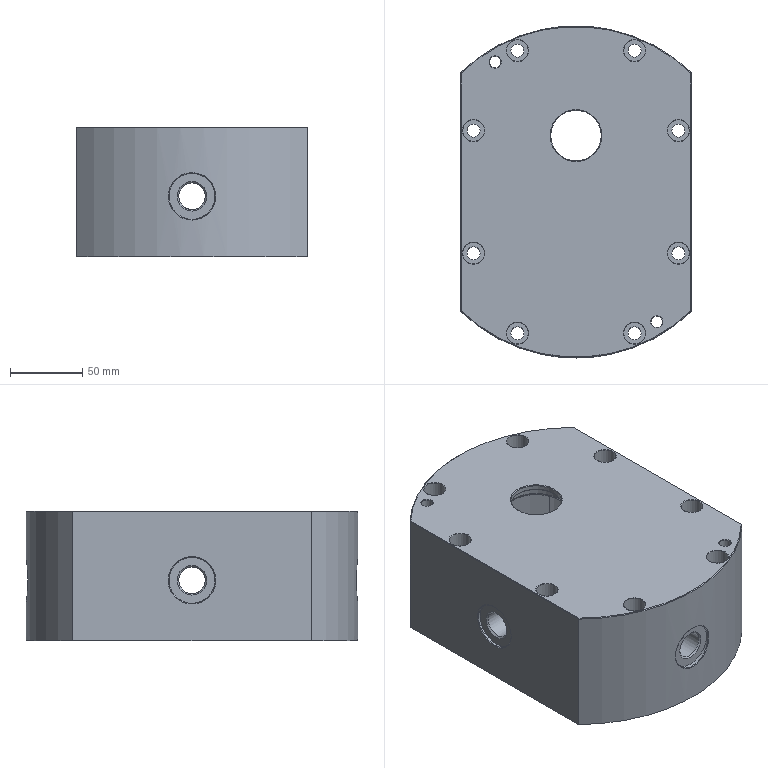NC program | NX | posted with a generic post | part box 160 x 230 x 90 mm
Whole program, first 1056 of 1320 lines:
N10 G17 G21 G94 G90
(HOLE_MILLING_COPY_COPY , TOOL : D10)
N12 T10 M6
N14 G54
N16 G17 G0 G90 X-97.931 Y40.564 B0. C0. S3000 M3
N18 G43 Z30. H10
N20 Z0.5
N22 G94 G3 X-99.181 Y39.314 R1.25 F2200.
N24 X-97.931 Y38.064 R1.25
N26 X-97.931 Y38.064 Z0.28 I0. J2.5
N28 X-97.931 Y38.064 Z0.06 I0. J2.5
N30 X-97.931 Y38.064 Z-0.16 I0. J2.5
N32 X-97.931 Y38.064 Z-0.38 I0. J2.5
N34 X-97.931 Y38.064 Z-0.6 I0. J2.5
N36 X-97.931 Y38.064 Z-0.82 I0. J2.5
N38 X-97.931 Y38.064 Z-1.04 I0. J2.5
N40 X-97.931 Y38.064 Z-1.26 I0. J2.5
N42 X-97.931 Y38.064 Z-1.48 I0. J2.5
N44 X-97.931 Y38.064 Z-1.7 I0. J2.5
N46 X-97.931 Y38.064 Z-1.92 I0. J2.5
N48 X-97.931 Y38.064 Z-2.14 I0. J2.5
N50 X-97.931 Y38.064 Z-2.36 I0. J2.5
N52 X-97.931 Y38.064 Z-2.58 I0. J2.5
N54 X-97.931 Y38.064 Z-2.8 I0. J2.5
N56 X-97.931 Y38.064 Z-3.02 I0. J2.5
N58 X-97.931 Y38.064 Z-3.24 I0. J2.5
N60 X-97.931 Y38.064 Z-3.46 I0. J2.5
N62 X-97.931 Y38.064 Z-3.68 I0. J2.5
N64 X-97.931 Y38.064 Z-3.9 I0. J2.5
N66 X-97.931 Y38.064 Z-4.12 I0. J2.5
N68 X-97.931 Y38.064 Z-4.34 I0. J2.5
N70 X-97.931 Y38.064 Z-4.56 I0. J2.5
N72 X-97.931 Y38.064 Z-4.78 I0. J2.5
N74 X-97.931 Y38.064 Z-5. I0. J2.5
N76 X-97.931 Y38.064 Z-5.22 I0. J2.5
N78 X-97.931 Y38.064 Z-5.44 I0. J2.5
N80 X-97.931 Y38.064 Z-5.66 I0. J2.5
N82 X-97.931 Y38.064 Z-5.88 I0. J2.5
N84 X-97.931 Y38.064 Z-6.1 I0. J2.5
N86 X-97.931 Y38.064 Z-6.32 I0. J2.5
N88 X-97.931 Y38.064 Z-6.54 I0. J2.5
N90 X-97.931 Y38.064 Z-6.76 I0. J2.5
N92 X-97.931 Y38.064 Z-6.98 I0. J2.5
N94 X-97.931 Y38.064 Z-7.2 I0. J2.5
N96 X-97.931 Y38.064 Z-7.42 I0. J2.5
N98 X-97.931 Y38.064 Z-7.64 I0. J2.5
N100 X-97.931 Y38.064 Z-7.86 I0. J2.5
N102 X-97.931 Y38.064 Z-8.08 I0. J2.5
N104 X-97.931 Y38.064 Z-8.3 I0. J2.5
N106 X-97.931 Y38.064 Z-8.52 I0. J2.5
N108 X-97.931 Y38.064 Z-8.74 I0. J2.5
N110 X-97.931 Y38.064 Z-8.96 I0. J2.5
N112 X-97.931 Y38.064 Z-9.18 I0. J2.5
N114 X-97.931 Y38.064 Z-9.4 I0. J2.5
N116 X-97.931 Y38.064 Z-9.62 I0. J2.5
N118 X-97.931 Y38.064 Z-9.84 I0. J2.5
N120 X-97.931 Y38.064 Z-10.06 I0. J2.5
N122 X-97.931 Y38.064 Z-10.28 I0. J2.5
N124 X-97.931 Y38.064 Z-10.5 I0. J2.5
N126 X-97.931 Y38.064 Z-10.72 I0. J2.5
N128 X-97.931 Y38.064 Z-10.94 I0. J2.5
N130 X-97.931 Y38.064 Z-11.16 I0. J2.5
N132 X-97.931 Y38.064 Z-11.38 I0. J2.5
N134 X-97.931 Y38.064 Z-11.6 I0. J2.5
N136 X-97.931 Y38.064 Z-11.82 I0. J2.5
N138 X-97.931 Y38.064 Z-12.04 I0. J2.5
N140 X-97.931 Y38.064 Z-12.26 I0. J2.5
N142 X-97.931 Y38.064 Z-12.48 I0. J2.5
N144 X-97.931 Y38.064 Z-12.7 I0. J2.5
N146 X-97.931 Y38.064 Z-12.92 I0. J2.5
N148 X-97.931 Y38.064 Z-13.14 I0. J2.5
N150 X-97.931 Y38.064 Z-13.36 I0. J2.5
N152 X-97.931 Y38.064 Z-13.58 I0. J2.5
N154 X-97.931 Y38.064 Z-13.8 I0. J2.5
N156 X-97.931 Y38.064 Z-14.02 I0. J2.5
N158 X-97.931 Y38.064 Z-14.24 I0. J2.5
N160 X-97.931 Y38.064 Z-14.46 I0. J2.5
N162 X-97.931 Y38.064 Z-14.68 I0. J2.5
N164 X-97.931 Y38.064 Z-14.9 I0. J2.5
N166 X-97.931 Y38.064 Z-15.12 I0. J2.5
N168 X-97.931 Y38.064 Z-15.34 I0. J2.5
N170 X-97.931 Y38.064 Z-15.56 I0. J2.5
N172 X-97.931 Y38.064 Z-15.78 I0. J2.5
N174 X-97.931 Y38.064 Z-16. I0. J2.5
N176 X-97.931 Y38.064 Z-16.22 I0. J2.5
N178 X-97.931 Y38.064 Z-16.44 I0. J2.5
N180 X-97.931 Y38.064 Z-16.66 I0. J2.5
N182 X-97.931 Y38.064 Z-16.88 I0. J2.5
N184 X-97.931 Y38.064 Z-17.1 I0. J2.5
N186 X-97.931 Y38.064 Z-17.32 I0. J2.5
N188 X-97.931 Y38.064 Z-17.54 I0. J2.5
N190 X-97.931 Y38.064 Z-17.76 I0. J2.5
N192 X-97.931 Y38.064 Z-17.98 I0. J2.5
N194 X-97.931 Y38.064 Z-18.2 I0. J2.5
N196 X-97.931 Y38.064 Z-18.42 I0. J2.5
N198 X-97.931 Y38.064 Z-18.64 I0. J2.5
N200 X-97.931 Y38.064 Z-18.86 I0. J2.5
N202 X-97.931 Y38.064 Z-19.08 I0. J2.5
N204 X-97.931 Y38.064 Z-19.3 I0. J2.5
N206 X-97.931 Y38.064 Z-19.52 I0. J2.5
N208 X-97.931 Y38.064 Z-19.74 I0. J2.5
N210 X-97.931 Y38.064 Z-19.96 I0. J2.5
N212 X-97.931 Y38.064 Z-20.18 I0. J2.5
N214 X-97.931 Y38.064 Z-20.4 I0. J2.5
N216 X-97.931 Y38.064 Z-20.62 I0. J2.5
N218 X-97.931 Y38.064 Z-20.84 I0. J2.5
N220 X-97.931 Y38.064 Z-21.06 I0. J2.5
N222 X-97.931 Y38.064 Z-21.28 I0. J2.5
N224 X-97.931 Y38.064 Z-21.5 I0. J2.5
N226 X-97.931 Y38.064 Z-21.72 I0. J2.5
N228 X-97.931 Y38.064 Z-21.94 I0. J2.5
N230 X-97.931 Y38.064 Z-22.16 I0. J2.5
N232 X-97.931 Y38.064 Z-22.38 I0. J2.5
N234 X-97.931 Y38.064 Z-22.6 I0. J2.5
N236 X-97.931 Y38.064 Z-22.82 I0. J2.5
N238 X-97.931 Y38.064 Z-23.04 I0. J2.5
N240 X-97.931 Y38.064 Z-23.26 I0. J2.5
N242 X-97.931 Y38.064 Z-23.48 I0. J2.5
N244 X-97.931 Y38.064 Z-23.7 I0. J2.5
N246 X-97.931 Y38.064 Z-23.92 I0. J2.5
N248 X-97.931 Y38.064 Z-24.14 I0. J2.5
N250 X-97.931 Y38.064 Z-24.36 I0. J2.5
N252 X-97.931 Y38.064 Z-24.58 I0. J2.5
N254 X-97.931 Y38.064 Z-24.8 I0. J2.5
N256 X-99.283 Y38.461 Z-25. R-2.5
N258 X-95.828 Y39.213 R2.5
N260 X-99.283 Y38.461 R-2.5
N262 X-97.555 Y38.837 R1.25
N264 X-97.931 Y40.564 R1.25
N266 G0 Z30.
N268 X-42.5 Y71.
N270 Z0.5
N272 G3 X-43.75 Y69.75 R1.25
N274 X-42.5 Y68.5 R1.25
N276 X-42.5 Y68.5 Z0.28 I0. J2.5
N278 X-42.5 Y68.5 Z0.06 I0. J2.5
N280 X-42.5 Y68.5 Z-0.16 I0. J2.5
N282 X-42.5 Y68.5 Z-0.38 I0. J2.5
N284 X-42.5 Y68.5 Z-0.6 I0. J2.5
N286 X-42.5 Y68.5 Z-0.82 I0. J2.5
N288 X-42.5 Y68.5 Z-1.04 I0. J2.5
N290 X-42.5 Y68.5 Z-1.26 I0. J2.5
N292 X-42.5 Y68.5 Z-1.48 I0. J2.5
N294 X-42.5 Y68.5 Z-1.7 I0. J2.5
N296 X-42.5 Y68.5 Z-1.92 I0. J2.5
N298 X-42.5 Y68.5 Z-2.14 I0. J2.5
N300 X-42.5 Y68.5 Z-2.36 I0. J2.5
N302 X-42.5 Y68.5 Z-2.58 I0. J2.5
N304 X-42.5 Y68.5 Z-2.8 I0. J2.5
N306 X-42.5 Y68.5 Z-3.02 I0. J2.5
N308 X-42.5 Y68.5 Z-3.24 I0. J2.5
N310 X-42.5 Y68.5 Z-3.46 I0. J2.5
N312 X-42.5 Y68.5 Z-3.68 I0. J2.5
N314 X-42.5 Y68.5 Z-3.9 I0. J2.5
N316 X-42.5 Y68.5 Z-4.12 I0. J2.5
N318 X-42.5 Y68.5 Z-4.34 I0. J2.5
N320 X-42.5 Y68.5 Z-4.56 I0. J2.5
N322 X-42.5 Y68.5 Z-4.78 I0. J2.5
N324 X-42.5 Y68.5 Z-5. I0. J2.5
N326 X-42.5 Y68.5 Z-5.22 I0. J2.5
N328 X-42.5 Y68.5 Z-5.44 I0. J2.5
N330 X-42.5 Y68.5 Z-5.66 I0. J2.5
N332 X-42.5 Y68.5 Z-5.88 I0. J2.5
N334 X-42.5 Y68.5 Z-6.1 I0. J2.5
N336 X-42.5 Y68.5 Z-6.32 I0. J2.5
N338 X-42.5 Y68.5 Z-6.54 I0. J2.5
N340 X-42.5 Y68.5 Z-6.76 I0. J2.5
N342 X-42.5 Y68.5 Z-6.98 I0. J2.5
N344 X-42.5 Y68.5 Z-7.2 I0. J2.5
N346 X-42.5 Y68.5 Z-7.42 I0. J2.5
N348 X-42.5 Y68.5 Z-7.64 I0. J2.5
N350 X-42.5 Y68.5 Z-7.86 I0. J2.5
N352 X-42.5 Y68.5 Z-8.08 I0. J2.5
N354 X-42.5 Y68.5 Z-8.3 I0. J2.5
N356 X-42.5 Y68.5 Z-8.52 I0. J2.5
N358 X-42.5 Y68.5 Z-8.74 I0. J2.5
N360 X-42.5 Y68.5 Z-8.96 I0. J2.5
N362 X-42.5 Y68.5 Z-9.18 I0. J2.5
N364 X-42.5 Y68.5 Z-9.4 I0. J2.5
N366 X-42.5 Y68.5 Z-9.62 I0. J2.5
N368 X-42.5 Y68.5 Z-9.84 I0. J2.5
N370 X-42.5 Y68.5 Z-10.06 I0. J2.5
N372 X-42.5 Y68.5 Z-10.28 I0. J2.5
N374 X-42.5 Y68.5 Z-10.5 I0. J2.5
N376 X-42.5 Y68.5 Z-10.72 I0. J2.5
N378 X-42.5 Y68.5 Z-10.94 I0. J2.5
N380 X-42.5 Y68.5 Z-11.16 I0. J2.5
N382 X-42.5 Y68.5 Z-11.38 I0. J2.5
N384 X-42.5 Y68.5 Z-11.6 I0. J2.5
N386 X-42.5 Y68.5 Z-11.82 I0. J2.5
N388 X-42.5 Y68.5 Z-12.04 I0. J2.5
N390 X-42.5 Y68.5 Z-12.26 I0. J2.5
N392 X-42.5 Y68.5 Z-12.48 I0. J2.5
N394 X-42.5 Y68.5 Z-12.7 I0. J2.5
N396 X-42.5 Y68.5 Z-12.92 I0. J2.5
N398 X-42.5 Y68.5 Z-13.14 I0. J2.5
N400 X-42.5 Y68.5 Z-13.36 I0. J2.5
N402 X-42.5 Y68.5 Z-13.58 I0. J2.5
N404 X-42.5 Y68.5 Z-13.8 I0. J2.5
N406 X-42.5 Y68.5 Z-14.02 I0. J2.5
N408 X-42.5 Y68.5 Z-14.24 I0. J2.5
N410 X-42.5 Y68.5 Z-14.46 I0. J2.5
N412 X-42.5 Y68.5 Z-14.68 I0. J2.5
N414 X-42.5 Y68.5 Z-14.9 I0. J2.5
N416 X-42.5 Y68.5 Z-15.12 I0. J2.5
N418 X-42.5 Y68.5 Z-15.34 I0. J2.5
N420 X-42.5 Y68.5 Z-15.56 I0. J2.5
N422 X-42.5 Y68.5 Z-15.78 I0. J2.5
N424 X-42.5 Y68.5 Z-16. I0. J2.5
N426 X-42.5 Y68.5 Z-16.22 I0. J2.5
N428 X-42.5 Y68.5 Z-16.44 I0. J2.5
N430 X-42.5 Y68.5 Z-16.66 I0. J2.5
N432 X-42.5 Y68.5 Z-16.88 I0. J2.5
N434 X-42.5 Y68.5 Z-17.1 I0. J2.5
N436 X-42.5 Y68.5 Z-17.32 I0. J2.5
N438 X-42.5 Y68.5 Z-17.54 I0. J2.5
N440 X-42.5 Y68.5 Z-17.76 I0. J2.5
N442 X-42.5 Y68.5 Z-17.98 I0. J2.5
N444 X-42.5 Y68.5 Z-18.2 I0. J2.5
N446 X-42.5 Y68.5 Z-18.42 I0. J2.5
N448 X-42.5 Y68.5 Z-18.64 I0. J2.5
N450 X-42.5 Y68.5 Z-18.86 I0. J2.5
N452 X-42.5 Y68.5 Z-19.08 I0. J2.5
N454 X-42.5 Y68.5 Z-19.3 I0. J2.5
N456 X-42.5 Y68.5 Z-19.52 I0. J2.5
N458 X-42.5 Y68.5 Z-19.74 I0. J2.5
N460 X-42.5 Y68.5 Z-19.96 I0. J2.5
N462 X-42.5 Y68.5 Z-20.18 I0. J2.5
N464 X-42.5 Y68.5 Z-20.4 I0. J2.5
N466 X-42.5 Y68.5 Z-20.62 I0. J2.5
N468 X-42.5 Y68.5 Z-20.84 I0. J2.5
N470 X-42.5 Y68.5 Z-21.06 I0. J2.5
N472 X-42.5 Y68.5 Z-21.28 I0. J2.5
N474 X-42.5 Y68.5 Z-21.5 I0. J2.5
N476 X-42.5 Y68.5 Z-21.72 I0. J2.5
N478 X-42.5 Y68.5 Z-21.94 I0. J2.5
N480 X-42.5 Y68.5 Z-22.16 I0. J2.5
N482 X-42.5 Y68.5 Z-22.38 I0. J2.5
N484 X-42.5 Y68.5 Z-22.6 I0. J2.5
N486 X-42.5 Y68.5 Z-22.82 I0. J2.5
N488 X-42.5 Y68.5 Z-23.04 I0. J2.5
N490 X-42.5 Y68.5 Z-23.26 I0. J2.5
N492 X-42.5 Y68.5 Z-23.48 I0. J2.5
N494 X-42.5 Y68.5 Z-23.7 I0. J2.5
N496 X-42.5 Y68.5 Z-23.92 I0. J2.5
N498 X-42.5 Y68.5 Z-24.14 I0. J2.5
N500 X-42.5 Y68.5 Z-24.36 I0. J2.5
N502 X-42.5 Y68.5 Z-24.58 I0. J2.5
N504 X-42.5 Y68.5 Z-24.8 I0. J2.5
N506 X-43.852 Y68.897 Z-25. R-2.5
N508 X-40.397 Y69.648 R2.5
N510 X-43.852 Y68.897 R-2.5
N512 X-42.124 Y69.273 R1.25
N514 X-42.5 Y71. R1.25
N516 G0 Z30.
N518 X42.5
N520 Z0.5
N522 G3 X41.25 Y69.75 R1.25
N524 X42.5 Y68.5 R1.25
N526 X42.5 Y68.5 Z0.28 I0. J2.5
N528 X42.5 Y68.5 Z0.06 I0. J2.5
N530 X42.5 Y68.5 Z-0.16 I0. J2.5
N532 X42.5 Y68.5 Z-0.38 I0. J2.5
N534 X42.5 Y68.5 Z-0.6 I0. J2.5
N536 X42.5 Y68.5 Z-0.82 I0. J2.5
N538 X42.5 Y68.5 Z-1.04 I0. J2.5
N540 X42.5 Y68.5 Z-1.26 I0. J2.5
N542 X42.5 Y68.5 Z-1.48 I0. J2.5
N544 X42.5 Y68.5 Z-1.7 I0. J2.5
N546 X42.5 Y68.5 Z-1.92 I0. J2.5
N548 X42.5 Y68.5 Z-2.14 I0. J2.5
N550 X42.5 Y68.5 Z-2.36 I0. J2.5
N552 X42.5 Y68.5 Z-2.58 I0. J2.5
N554 X42.5 Y68.5 Z-2.8 I0. J2.5
N556 X42.5 Y68.5 Z-3.02 I0. J2.5
N558 X42.5 Y68.5 Z-3.24 I0. J2.5
N560 X42.5 Y68.5 Z-3.46 I0. J2.5
N562 X42.5 Y68.5 Z-3.68 I0. J2.5
N564 X42.5 Y68.5 Z-3.9 I0. J2.5
N566 X42.5 Y68.5 Z-4.12 I0. J2.5
N568 X42.5 Y68.5 Z-4.34 I0. J2.5
N570 X42.5 Y68.5 Z-4.56 I0. J2.5
N572 X42.5 Y68.5 Z-4.78 I0. J2.5
N574 X42.5 Y68.5 Z-5. I0. J2.5
N576 X42.5 Y68.5 Z-5.22 I0. J2.5
N578 X42.5 Y68.5 Z-5.44 I0. J2.5
N580 X42.5 Y68.5 Z-5.66 I0. J2.5
N582 X42.5 Y68.5 Z-5.88 I0. J2.5
N584 X42.5 Y68.5 Z-6.1 I0. J2.5
N586 X42.5 Y68.5 Z-6.32 I0. J2.5
N588 X42.5 Y68.5 Z-6.54 I0. J2.5
N590 X42.5 Y68.5 Z-6.76 I0. J2.5
N592 X42.5 Y68.5 Z-6.98 I0. J2.5
N594 X42.5 Y68.5 Z-7.2 I0. J2.5
N596 X42.5 Y68.5 Z-7.42 I0. J2.5
N598 X42.5 Y68.5 Z-7.64 I0. J2.5
N600 X42.5 Y68.5 Z-7.86 I0. J2.5
N602 X42.5 Y68.5 Z-8.08 I0. J2.5
N604 X42.5 Y68.5 Z-8.3 I0. J2.5
N606 X42.5 Y68.5 Z-8.52 I0. J2.5
N608 X42.5 Y68.5 Z-8.74 I0. J2.5
N610 X42.5 Y68.5 Z-8.96 I0. J2.5
N612 X42.5 Y68.5 Z-9.18 I0. J2.5
N614 X42.5 Y68.5 Z-9.4 I0. J2.5
N616 X42.5 Y68.5 Z-9.62 I0. J2.5
N618 X42.5 Y68.5 Z-9.84 I0. J2.5
N620 X42.5 Y68.5 Z-10.06 I0. J2.5
N622 X42.5 Y68.5 Z-10.28 I0. J2.5
N624 X42.5 Y68.5 Z-10.5 I0. J2.5
N626 X42.5 Y68.5 Z-10.72 I0. J2.5
N628 X42.5 Y68.5 Z-10.94 I0. J2.5
N630 X42.5 Y68.5 Z-11.16 I0. J2.5
N632 X42.5 Y68.5 Z-11.38 I0. J2.5
N634 X42.5 Y68.5 Z-11.6 I0. J2.5
N636 X42.5 Y68.5 Z-11.82 I0. J2.5
N638 X42.5 Y68.5 Z-12.04 I0. J2.5
N640 X42.5 Y68.5 Z-12.26 I0. J2.5
N642 X42.5 Y68.5 Z-12.48 I0. J2.5
N644 X42.5 Y68.5 Z-12.7 I0. J2.5
N646 X42.5 Y68.5 Z-12.92 I0. J2.5
N648 X42.5 Y68.5 Z-13.14 I0. J2.5
N650 X42.5 Y68.5 Z-13.36 I0. J2.5
N652 X42.5 Y68.5 Z-13.58 I0. J2.5
N654 X42.5 Y68.5 Z-13.8 I0. J2.5
N656 X42.5 Y68.5 Z-14.02 I0. J2.5
N658 X42.5 Y68.5 Z-14.24 I0. J2.5
N660 X42.5 Y68.5 Z-14.46 I0. J2.5
N662 X42.5 Y68.5 Z-14.68 I0. J2.5
N664 X42.5 Y68.5 Z-14.9 I0. J2.5
N666 X42.5 Y68.5 Z-15.12 I0. J2.5
N668 X42.5 Y68.5 Z-15.34 I0. J2.5
N670 X42.5 Y68.5 Z-15.56 I0. J2.5
N672 X42.5 Y68.5 Z-15.78 I0. J2.5
N674 X42.5 Y68.5 Z-16. I0. J2.5
N676 X42.5 Y68.5 Z-16.22 I0. J2.5
N678 X42.5 Y68.5 Z-16.44 I0. J2.5
N680 X42.5 Y68.5 Z-16.66 I0. J2.5
N682 X42.5 Y68.5 Z-16.88 I0. J2.5
N684 X42.5 Y68.5 Z-17.1 I0. J2.5
N686 X42.5 Y68.5 Z-17.32 I0. J2.5
N688 X42.5 Y68.5 Z-17.54 I0. J2.5
N690 X42.5 Y68.5 Z-17.76 I0. J2.5
N692 X42.5 Y68.5 Z-17.98 I0. J2.5
N694 X42.5 Y68.5 Z-18.2 I0. J2.5
N696 X42.5 Y68.5 Z-18.42 I0. J2.5
N698 X42.5 Y68.5 Z-18.64 I0. J2.5
N700 X42.5 Y68.5 Z-18.86 I0. J2.5
N702 X42.5 Y68.5 Z-19.08 I0. J2.5
N704 X42.5 Y68.5 Z-19.3 I0. J2.5
N706 X42.5 Y68.5 Z-19.52 I0. J2.5
N708 X42.5 Y68.5 Z-19.74 I0. J2.5
N710 X42.5 Y68.5 Z-19.96 I0. J2.5
N712 X42.5 Y68.5 Z-20.18 I0. J2.5
N714 X42.5 Y68.5 Z-20.4 I0. J2.5
N716 X42.5 Y68.5 Z-20.62 I0. J2.5
N718 X42.5 Y68.5 Z-20.84 I0. J2.5
N720 X42.5 Y68.5 Z-21.06 I0. J2.5
N722 X42.5 Y68.5 Z-21.28 I0. J2.5
N724 X42.5 Y68.5 Z-21.5 I0. J2.5
N726 X42.5 Y68.5 Z-21.72 I0. J2.5
N728 X42.5 Y68.5 Z-21.94 I0. J2.5
N730 X42.5 Y68.5 Z-22.16 I0. J2.5
N732 X42.5 Y68.5 Z-22.38 I0. J2.5
N734 X42.5 Y68.5 Z-22.6 I0. J2.5
N736 X42.5 Y68.5 Z-22.82 I0. J2.5
N738 X42.5 Y68.5 Z-23.04 I0. J2.5
N740 X42.5 Y68.5 Z-23.26 I0. J2.5
N742 X42.5 Y68.5 Z-23.48 I0. J2.5
N744 X42.5 Y68.5 Z-23.7 I0. J2.5
N746 X42.5 Y68.5 Z-23.92 I0. J2.5
N748 X42.5 Y68.5 Z-24.14 I0. J2.5
N750 X42.5 Y68.5 Z-24.36 I0. J2.5
N752 X42.5 Y68.5 Z-24.58 I0. J2.5
N754 X42.5 Y68.5 Z-24.8 I0. J2.5
N756 X41.148 Y68.897 Z-25. R-2.5
N758 X44.603 Y69.648 R2.5
N760 X41.148 Y68.897 R-2.5
N762 X42.876 Y69.273 R1.25
N764 X42.5 Y71. R1.25
N766 G0 Z30.
N768 X97.931 Y40.564
N770 Z0.5
N772 G3 X96.681 Y39.314 R1.25
N774 X97.931 Y38.064 R1.25
N776 X97.931 Y38.064 Z0.28 I0. J2.5
N778 X97.931 Y38.064 Z0.06 I0. J2.5
N780 X97.931 Y38.064 Z-0.16 I0. J2.5
N782 X97.931 Y38.064 Z-0.38 I0. J2.5
N784 X97.931 Y38.064 Z-0.6 I0. J2.5
N786 X97.931 Y38.064 Z-0.82 I0. J2.5
N788 X97.931 Y38.064 Z-1.04 I0. J2.5
N790 X97.931 Y38.064 Z-1.26 I0. J2.5
N792 X97.931 Y38.064 Z-1.48 I0. J2.5
N794 X97.931 Y38.064 Z-1.7 I0. J2.5
N796 X97.931 Y38.064 Z-1.92 I0. J2.5
N798 X97.931 Y38.064 Z-2.14 I0. J2.5
N800 X97.931 Y38.064 Z-2.36 I0. J2.5
N802 X97.931 Y38.064 Z-2.58 I0. J2.5
N804 X97.931 Y38.064 Z-2.8 I0. J2.5
N806 X97.931 Y38.064 Z-3.02 I0. J2.5
N808 X97.931 Y38.064 Z-3.24 I0. J2.5
N810 X97.931 Y38.064 Z-3.46 I0. J2.5
N812 X97.931 Y38.064 Z-3.68 I0. J2.5
N814 X97.931 Y38.064 Z-3.9 I0. J2.5
N816 X97.931 Y38.064 Z-4.12 I0. J2.5
N818 X97.931 Y38.064 Z-4.34 I0. J2.5
N820 X97.931 Y38.064 Z-4.56 I0. J2.5
N822 X97.931 Y38.064 Z-4.78 I0. J2.5
N824 X97.931 Y38.064 Z-5. I0. J2.5
N826 X97.931 Y38.064 Z-5.22 I0. J2.5
N828 X97.931 Y38.064 Z-5.44 I0. J2.5
N830 X97.931 Y38.064 Z-5.66 I0. J2.5
N832 X97.931 Y38.064 Z-5.88 I0. J2.5
N834 X97.931 Y38.064 Z-6.1 I0. J2.5
N836 X97.931 Y38.064 Z-6.32 I0. J2.5
N838 X97.931 Y38.064 Z-6.54 I0. J2.5
N840 X97.931 Y38.064 Z-6.76 I0. J2.5
N842 X97.931 Y38.064 Z-6.98 I0. J2.5
N844 X97.931 Y38.064 Z-7.2 I0. J2.5
N846 X97.931 Y38.064 Z-7.42 I0. J2.5
N848 X97.931 Y38.064 Z-7.64 I0. J2.5
N850 X97.931 Y38.064 Z-7.86 I0. J2.5
N852 X97.931 Y38.064 Z-8.08 I0. J2.5
N854 X97.931 Y38.064 Z-8.3 I0. J2.5
N856 X97.931 Y38.064 Z-8.52 I0. J2.5
N858 X97.931 Y38.064 Z-8.74 I0. J2.5
N860 X97.931 Y38.064 Z-8.96 I0. J2.5
N862 X97.931 Y38.064 Z-9.18 I0. J2.5
N864 X97.931 Y38.064 Z-9.4 I0. J2.5
N866 X97.931 Y38.064 Z-9.62 I0. J2.5
N868 X97.931 Y38.064 Z-9.84 I0. J2.5
N870 X97.931 Y38.064 Z-10.06 I0. J2.5
N872 X97.931 Y38.064 Z-10.28 I0. J2.5
N874 X97.931 Y38.064 Z-10.5 I0. J2.5
N876 X97.931 Y38.064 Z-10.72 I0. J2.5
N878 X97.931 Y38.064 Z-10.94 I0. J2.5
N880 X97.931 Y38.064 Z-11.16 I0. J2.5
N882 X97.931 Y38.064 Z-11.38 I0. J2.5
N884 X97.931 Y38.064 Z-11.6 I0. J2.5
N886 X97.931 Y38.064 Z-11.82 I0. J2.5
N888 X97.931 Y38.064 Z-12.04 I0. J2.5
N890 X97.931 Y38.064 Z-12.26 I0. J2.5
N892 X97.931 Y38.064 Z-12.48 I0. J2.5
N894 X97.931 Y38.064 Z-12.7 I0. J2.5
N896 X97.931 Y38.064 Z-12.92 I0. J2.5
N898 X97.931 Y38.064 Z-13.14 I0. J2.5
N900 X97.931 Y38.064 Z-13.36 I0. J2.5
N902 X97.931 Y38.064 Z-13.58 I0. J2.5
N904 X97.931 Y38.064 Z-13.8 I0. J2.5
N906 X97.931 Y38.064 Z-14.02 I0. J2.5
N908 X97.931 Y38.064 Z-14.24 I0. J2.5
N910 X97.931 Y38.064 Z-14.46 I0. J2.5
N912 X97.931 Y38.064 Z-14.68 I0. J2.5
N914 X97.931 Y38.064 Z-14.9 I0. J2.5
N916 X97.931 Y38.064 Z-15.12 I0. J2.5
N918 X97.931 Y38.064 Z-15.34 I0. J2.5
N920 X97.931 Y38.064 Z-15.56 I0. J2.5
N922 X97.931 Y38.064 Z-15.78 I0. J2.5
N924 X97.931 Y38.064 Z-16. I0. J2.5
N926 X97.931 Y38.064 Z-16.22 I0. J2.5
N928 X97.931 Y38.064 Z-16.44 I0. J2.5
N930 X97.931 Y38.064 Z-16.66 I0. J2.5
N932 X97.931 Y38.064 Z-16.88 I0. J2.5
N934 X97.931 Y38.064 Z-17.1 I0. J2.5
N936 X97.931 Y38.064 Z-17.32 I0. J2.5
N938 X97.931 Y38.064 Z-17.54 I0. J2.5
N940 X97.931 Y38.064 Z-17.76 I0. J2.5
N942 X97.931 Y38.064 Z-17.98 I0. J2.5
N944 X97.931 Y38.064 Z-18.2 I0. J2.5
N946 X97.931 Y38.064 Z-18.42 I0. J2.5
N948 X97.931 Y38.064 Z-18.64 I0. J2.5
N950 X97.931 Y38.064 Z-18.86 I0. J2.5
N952 X97.931 Y38.064 Z-19.08 I0. J2.5
N954 X97.931 Y38.064 Z-19.3 I0. J2.5
N956 X97.931 Y38.064 Z-19.52 I0. J2.5
N958 X97.931 Y38.064 Z-19.74 I0. J2.5
N960 X97.931 Y38.064 Z-19.96 I0. J2.5
N962 X97.931 Y38.064 Z-20.18 I0. J2.5
N964 X97.931 Y38.064 Z-20.4 I0. J2.5
N966 X97.931 Y38.064 Z-20.62 I0. J2.5
N968 X97.931 Y38.064 Z-20.84 I0. J2.5
N970 X97.931 Y38.064 Z-21.06 I0. J2.5
N972 X97.931 Y38.064 Z-21.28 I0. J2.5
N974 X97.931 Y38.064 Z-21.5 I0. J2.5
N976 X97.931 Y38.064 Z-21.72 I0. J2.5
N978 X97.931 Y38.064 Z-21.94 I0. J2.5
N980 X97.931 Y38.064 Z-22.16 I0. J2.5
N982 X97.931 Y38.064 Z-22.38 I0. J2.5
N984 X97.931 Y38.064 Z-22.6 I0. J2.5
N986 X97.931 Y38.064 Z-22.82 I0. J2.5
N988 X97.931 Y38.064 Z-23.04 I0. J2.5
N990 X97.931 Y38.064 Z-23.26 I0. J2.5
N992 X97.931 Y38.064 Z-23.48 I0. J2.5
N994 X97.931 Y38.064 Z-23.7 I0. J2.5
N996 X97.931 Y38.064 Z-23.92 I0. J2.5
N998 X97.931 Y38.064 Z-24.14 I0. J2.5
N1000 X97.931 Y38.064 Z-24.36 I0. J2.5
N1002 X97.931 Y38.064 Z-24.58 I0. J2.5
N1004 X97.931 Y38.064 Z-24.8 I0. J2.5
N1006 X96.58 Y38.461 Z-25. R-2.5
N1008 X100.034 Y39.213 R2.5
N1010 X96.58 Y38.461 R-2.5
N1012 X98.307 Y38.837 R1.25
N1014 X97.931 Y40.564 R1.25
N1016 G0 Z30.
N1018 Y-40.564
N1020 Z0.5
N1022 G3 X96.681 Y-41.814 R1.25
N1024 X97.931 Y-43.064 R1.25
N1026 X97.931 Y-43.064 Z0.28 I0. J2.5
N1028 X97.931 Y-43.064 Z0.06 I0. J2.5
N1030 X97.931 Y-43.064 Z-0.16 I0. J2.5
N1032 X97.931 Y-43.064 Z-0.38 I0. J2.5
N1034 X97.931 Y-43.064 Z-0.6 I0. J2.5
N1036 X97.931 Y-43.064 Z-0.82 I0. J2.5
N1038 X97.931 Y-43.064 Z-1.04 I0. J2.5
N1040 X97.931 Y-43.064 Z-1.26 I0. J2.5
N1042 X97.931 Y-43.064 Z-1.48 I0. J2.5
N1044 X97.931 Y-43.064 Z-1.7 I0. J2.5
N1046 X97.931 Y-43.064 Z-1.92 I0. J2.5
N1048 X97.931 Y-43.064 Z-2.14 I0. J2.5
N1050 X97.931 Y-43.064 Z-2.36 I0. J2.5
N1052 X97.931 Y-43.064 Z-2.58 I0. J2.5
N1054 X97.931 Y-43.064 Z-2.8 I0. J2.5
N1056 X97.931 Y-43.064 Z-3.02 I0. J2.5
N1058 X97.931 Y-43.064 Z-3.24 I0. J2.5
N1060 X97.931 Y-43.064 Z-3.46 I0. J2.5
N1062 X97.931 Y-43.064 Z-3.68 I0. J2.5
N1064 X97.931 Y-43.064 Z-3.9 I0. J2.5
N1066 X97.931 Y-43.064 Z-4.12 I0. J2.5
N1068 X97.931 Y-43.064 Z-4.34 I0. J2.5
N1070 X97.931 Y-43.064 Z-4.56 I0. J2.5
N1072 X97.931 Y-43.064 Z-4.78 I0. J2.5
N1074 X97.931 Y-43.064 Z-5. I0. J2.5
N1076 X97.931 Y-43.064 Z-5.22 I0. J2.5
N1078 X97.931 Y-43.064 Z-5.44 I0. J2.5
N1080 X97.931 Y-43.064 Z-5.66 I0. J2.5
N1082 X97.931 Y-43.064 Z-5.88 I0. J2.5
N1084 X97.931 Y-43.064 Z-6.1 I0. J2.5
N1086 X97.931 Y-43.064 Z-6.32 I0. J2.5
N1088 X97.931 Y-43.064 Z-6.54 I0. J2.5
N1090 X97.931 Y-43.064 Z-6.76 I0. J2.5
N1092 X97.931 Y-43.064 Z-6.98 I0. J2.5
N1094 X97.931 Y-43.064 Z-7.2 I0. J2.5
N1096 X97.931 Y-43.064 Z-7.42 I0. J2.5
N1098 X97.931 Y-43.064 Z-7.64 I0. J2.5
N1100 X97.931 Y-43.064 Z-7.86 I0. J2.5
N1102 X97.931 Y-43.064 Z-8.08 I0. J2.5
N1104 X97.931 Y-43.064 Z-8.3 I0. J2.5
N1106 X97.931 Y-43.064 Z-8.52 I0. J2.5
N1108 X97.931 Y-43.064 Z-8.74 I0. J2.5
N1110 X97.931 Y-43.064 Z-8.96 I0. J2.5
N1112 X97.931 Y-43.064 Z-9.18 I0. J2.5
N1114 X97.931 Y-43.064 Z-9.4 I0. J2.5
N1116 X97.931 Y-43.064 Z-9.62 I0. J2.5
N1118 X97.931 Y-43.064 Z-9.84 I0. J2.5
N1120 X97.931 Y-43.064 Z-10.06 I0. J2.5
N1122 X97.931 Y-43.064 Z-10.28 I0. J2.5
N1124 X97.931 Y-43.064 Z-10.5 I0. J2.5
N1126 X97.931 Y-43.064 Z-10.72 I0. J2.5
N1128 X97.931 Y-43.064 Z-10.94 I0. J2.5
N1130 X97.931 Y-43.064 Z-11.16 I0. J2.5
N1132 X97.931 Y-43.064 Z-11.38 I0. J2.5
N1134 X97.931 Y-43.064 Z-11.6 I0. J2.5
N1136 X97.931 Y-43.064 Z-11.82 I0. J2.5
N1138 X97.931 Y-43.064 Z-12.04 I0. J2.5
N1140 X97.931 Y-43.064 Z-12.26 I0. J2.5
N1142 X97.931 Y-43.064 Z-12.48 I0. J2.5
N1144 X97.931 Y-43.064 Z-12.7 I0. J2.5
N1146 X97.931 Y-43.064 Z-12.92 I0. J2.5
N1148 X97.931 Y-43.064 Z-13.14 I0. J2.5
N1150 X97.931 Y-43.064 Z-13.36 I0. J2.5
N1152 X97.931 Y-43.064 Z-13.58 I0. J2.5
N1154 X97.931 Y-43.064 Z-13.8 I0. J2.5
N1156 X97.931 Y-43.064 Z-14.02 I0. J2.5
N1158 X97.931 Y-43.064 Z-14.24 I0. J2.5
N1160 X97.931 Y-43.064 Z-14.46 I0. J2.5
N1162 X97.931 Y-43.064 Z-14.68 I0. J2.5
N1164 X97.931 Y-43.064 Z-14.9 I0. J2.5
N1166 X97.931 Y-43.064 Z-15.12 I0. J2.5
N1168 X97.931 Y-43.064 Z-15.34 I0. J2.5
N1170 X97.931 Y-43.064 Z-15.56 I0. J2.5
N1172 X97.931 Y-43.064 Z-15.78 I0. J2.5
N1174 X97.931 Y-43.064 Z-16. I0. J2.5
N1176 X97.931 Y-43.064 Z-16.22 I0. J2.5
N1178 X97.931 Y-43.064 Z-16.44 I0. J2.5
N1180 X97.931 Y-43.064 Z-16.66 I0. J2.5
N1182 X97.931 Y-43.064 Z-16.88 I0. J2.5
N1184 X97.931 Y-43.064 Z-17.1 I0. J2.5
N1186 X97.931 Y-43.064 Z-17.32 I0. J2.5
N1188 X97.931 Y-43.064 Z-17.54 I0. J2.5
N1190 X97.931 Y-43.064 Z-17.76 I0. J2.5
N1192 X97.931 Y-43.064 Z-17.98 I0. J2.5
N1194 X97.931 Y-43.064 Z-18.2 I0. J2.5
N1196 X97.931 Y-43.064 Z-18.42 I0. J2.5
N1198 X97.931 Y-43.064 Z-18.64 I0. J2.5
N1200 X97.931 Y-43.064 Z-18.86 I0. J2.5
N1202 X97.931 Y-43.064 Z-19.08 I0. J2.5
N1204 X97.931 Y-43.064 Z-19.3 I0. J2.5
N1206 X97.931 Y-43.064 Z-19.52 I0. J2.5
N1208 X97.931 Y-43.064 Z-19.74 I0. J2.5
N1210 X97.931 Y-43.064 Z-19.96 I0. J2.5
N1212 X97.931 Y-43.064 Z-20.18 I0. J2.5
N1214 X97.931 Y-43.064 Z-20.4 I0. J2.5
N1216 X97.931 Y-43.064 Z-20.62 I0. J2.5
N1218 X97.931 Y-43.064 Z-20.84 I0. J2.5
N1220 X97.931 Y-43.064 Z-21.06 I0. J2.5
N1222 X97.931 Y-43.064 Z-21.28 I0. J2.5
N1224 X97.931 Y-43.064 Z-21.5 I0. J2.5
N1226 X97.931 Y-43.064 Z-21.72 I0. J2.5
N1228 X97.931 Y-43.064 Z-21.94 I0. J2.5
N1230 X97.931 Y-43.064 Z-22.16 I0. J2.5
N1232 X97.931 Y-43.064 Z-22.38 I0. J2.5
N1234 X97.931 Y-43.064 Z-22.6 I0. J2.5
N1236 X97.931 Y-43.064 Z-22.82 I0. J2.5
N1238 X97.931 Y-43.064 Z-23.04 I0. J2.5
N1240 X97.931 Y-43.064 Z-23.26 I0. J2.5
N1242 X97.931 Y-43.064 Z-23.48 I0. J2.5
N1244 X97.931 Y-43.064 Z-23.7 I0. J2.5
N1246 X97.931 Y-43.064 Z-23.92 I0. J2.5
N1248 X97.931 Y-43.064 Z-24.14 I0. J2.5
N1250 X97.931 Y-43.064 Z-24.36 I0. J2.5
N1252 X97.931 Y-43.064 Z-24.58 I0. J2.5
N1254 X97.931 Y-43.064 Z-24.8 I0. J2.5
N1256 X96.58 Y-42.668 Z-25. R-2.5
N1258 X100.034 Y-41.916 R2.5
N1260 X96.58 Y-42.668 R-2.5
N1262 X98.307 Y-42.292 R1.25
N1264 X97.931 Y-40.564 R1.25
N1266 G0 Z30.
N1268 X42.5 Y-71.
N1270 Z0.5
N1272 G3 X41.25 Y-72.25 R1.25
N1274 X42.5 Y-73.5 R1.25
N1276 X42.5 Y-73.5 Z0.28 I0. J2.5
N1278 X42.5 Y-73.5 Z0.06 I0. J2.5
N1280 X42.5 Y-73.5 Z-0.16 I0. J2.5
N1282 X42.5 Y-73.5 Z-0.38 I0. J2.5
N1284 X42.5 Y-73.5 Z-0.6 I0. J2.5
N1286 X42.5 Y-73.5 Z-0.82 I0. J2.5
N1288 X42.5 Y-73.5 Z-1.04 I0. J2.5
N1290 X42.5 Y-73.5 Z-1.26 I0. J2.5
N1292 X42.5 Y-73.5 Z-1.48 I0. J2.5
N1294 X42.5 Y-73.5 Z-1.7 I0. J2.5
N1296 X42.5 Y-73.5 Z-1.92 I0. J2.5
N1298 X42.5 Y-73.5 Z-2.14 I0. J2.5
N1300 X42.5 Y-73.5 Z-2.36 I0. J2.5
N1302 X42.5 Y-73.5 Z-2.58 I0. J2.5
N1304 X42.5 Y-73.5 Z-2.8 I0. J2.5
N1306 X42.5 Y-73.5 Z-3.02 I0. J2.5
N1308 X42.5 Y-73.5 Z-3.24 I0. J2.5
N1310 X42.5 Y-73.5 Z-3.46 I0. J2.5
N1312 X42.5 Y-73.5 Z-3.68 I0. J2.5
N1314 X42.5 Y-73.5 Z-3.9 I0. J2.5
N1316 X42.5 Y-73.5 Z-4.12 I0. J2.5
N1318 X42.5 Y-73.5 Z-4.34 I0. J2.5
N1320 X42.5 Y-73.5 Z-4.56 I0. J2.5
N1322 X42.5 Y-73.5 Z-4.78 I0. J2.5
N1324 X42.5 Y-73.5 Z-5. I0. J2.5
N1326 X42.5 Y-73.5 Z-5.22 I0. J2.5
N1328 X42.5 Y-73.5 Z-5.44 I0. J2.5
N1330 X42.5 Y-73.5 Z-5.66 I0. J2.5
N1332 X42.5 Y-73.5 Z-5.88 I0. J2.5
N1334 X42.5 Y-73.5 Z-6.1 I0. J2.5
N1336 X42.5 Y-73.5 Z-6.32 I0. J2.5
N1338 X42.5 Y-73.5 Z-6.54 I0. J2.5
N1340 X42.5 Y-73.5 Z-6.76 I0. J2.5
N1342 X42.5 Y-73.5 Z-6.98 I0. J2.5
N1344 X42.5 Y-73.5 Z-7.2 I0. J2.5
N1346 X42.5 Y-73.5 Z-7.42 I0. J2.5
N1348 X42.5 Y-73.5 Z-7.64 I0. J2.5
N1350 X42.5 Y-73.5 Z-7.86 I0. J2.5
N1352 X42.5 Y-73.5 Z-8.08 I0. J2.5
N1354 X42.5 Y-73.5 Z-8.3 I0. J2.5
N1356 X42.5 Y-73.5 Z-8.52 I0. J2.5
N1358 X42.5 Y-73.5 Z-8.74 I0. J2.5
N1360 X42.5 Y-73.5 Z-8.96 I0. J2.5
N1362 X42.5 Y-73.5 Z-9.18 I0. J2.5
N1364 X42.5 Y-73.5 Z-9.4 I0. J2.5
N1366 X42.5 Y-73.5 Z-9.62 I0. J2.5
N1368 X42.5 Y-73.5 Z-9.84 I0. J2.5
N1370 X42.5 Y-73.5 Z-10.06 I0. J2.5
N1372 X42.5 Y-73.5 Z-10.28 I0. J2.5
N1374 X42.5 Y-73.5 Z-10.5 I0. J2.5
N1376 X42.5 Y-73.5 Z-10.72 I0. J2.5
N1378 X42.5 Y-73.5 Z-10.94 I0. J2.5
N1380 X42.5 Y-73.5 Z-11.16 I0. J2.5
N1382 X42.5 Y-73.5 Z-11.38 I0. J2.5
N1384 X42.5 Y-73.5 Z-11.6 I0. J2.5
N1386 X42.5 Y-73.5 Z-11.82 I0. J2.5
N1388 X42.5 Y-73.5 Z-12.04 I0. J2.5
N1390 X42.5 Y-73.5 Z-12.26 I0. J2.5
N1392 X42.5 Y-73.5 Z-12.48 I0. J2.5
N1394 X42.5 Y-73.5 Z-12.7 I0. J2.5
N1396 X42.5 Y-73.5 Z-12.92 I0. J2.5
N1398 X42.5 Y-73.5 Z-13.14 I0. J2.5
N1400 X42.5 Y-73.5 Z-13.36 I0. J2.5
N1402 X42.5 Y-73.5 Z-13.58 I0. J2.5
N1404 X42.5 Y-73.5 Z-13.8 I0. J2.5
N1406 X42.5 Y-73.5 Z-14.02 I0. J2.5
N1408 X42.5 Y-73.5 Z-14.24 I0. J2.5
N1410 X42.5 Y-73.5 Z-14.46 I0. J2.5
N1412 X42.5 Y-73.5 Z-14.68 I0. J2.5
N1414 X42.5 Y-73.5 Z-14.9 I0. J2.5
N1416 X42.5 Y-73.5 Z-15.12 I0. J2.5
N1418 X42.5 Y-73.5 Z-15.34 I0. J2.5
N1420 X42.5 Y-73.5 Z-15.56 I0. J2.5
N1422 X42.5 Y-73.5 Z-15.78 I0. J2.5
N1424 X42.5 Y-73.5 Z-16. I0. J2.5
N1426 X42.5 Y-73.5 Z-16.22 I0. J2.5
N1428 X42.5 Y-73.5 Z-16.44 I0. J2.5
N1430 X42.5 Y-73.5 Z-16.66 I0. J2.5
N1432 X42.5 Y-73.5 Z-16.88 I0. J2.5
N1434 X42.5 Y-73.5 Z-17.1 I0. J2.5
N1436 X42.5 Y-73.5 Z-17.32 I0. J2.5
N1438 X42.5 Y-73.5 Z-17.54 I0. J2.5
N1440 X42.5 Y-73.5 Z-17.76 I0. J2.5
N1442 X42.5 Y-73.5 Z-17.98 I0. J2.5
N1444 X42.5 Y-73.5 Z-18.2 I0. J2.5
N1446 X42.5 Y-73.5 Z-18.42 I0. J2.5
N1448 X42.5 Y-73.5 Z-18.64 I0. J2.5
N1450 X42.5 Y-73.5 Z-18.86 I0. J2.5
N1452 X42.5 Y-73.5 Z-19.08 I0. J2.5
N1454 X42.5 Y-73.5 Z-19.3 I0. J2.5
N1456 X42.5 Y-73.5 Z-19.52 I0. J2.5
N1458 X42.5 Y-73.5 Z-19.74 I0. J2.5
N1460 X42.5 Y-73.5 Z-19.96 I0. J2.5
N1462 X42.5 Y-73.5 Z-20.18 I0. J2.5
N1464 X42.5 Y-73.5 Z-20.4 I0. J2.5
N1466 X42.5 Y-73.5 Z-20.62 I0. J2.5
N1468 X42.5 Y-73.5 Z-20.84 I0. J2.5
N1470 X42.5 Y-73.5 Z-21.06 I0. J2.5
N1472 X42.5 Y-73.5 Z-21.28 I0. J2.5
N1474 X42.5 Y-73.5 Z-21.5 I0. J2.5
N1476 X42.5 Y-73.5 Z-21.72 I0. J2.5
N1478 X42.5 Y-73.5 Z-21.94 I0. J2.5
N1480 X42.5 Y-73.5 Z-22.16 I0. J2.5
N1482 X42.5 Y-73.5 Z-22.38 I0. J2.5
N1484 X42.5 Y-73.5 Z-22.6 I0. J2.5
N1486 X42.5 Y-73.5 Z-22.82 I0. J2.5
N1488 X42.5 Y-73.5 Z-23.04 I0. J2.5
N1490 X42.5 Y-73.5 Z-23.26 I0. J2.5
N1492 X42.5 Y-73.5 Z-23.48 I0. J2.5
N1494 X42.5 Y-73.5 Z-23.7 I0. J2.5
N1496 X42.5 Y-73.5 Z-23.92 I0. J2.5
N1498 X42.5 Y-73.5 Z-24.14 I0. J2.5
N1500 X42.5 Y-73.5 Z-24.36 I0. J2.5
N1502 X42.5 Y-73.5 Z-24.58 I0. J2.5
N1504 X42.5 Y-73.5 Z-24.8 I0. J2.5
N1506 X41.148 Y-73.103 Z-25. R-2.5
N1508 X44.603 Y-72.352 R2.5
N1510 X41.148 Y-73.103 R-2.5
N1512 X42.876 Y-72.727 R1.25
N1514 X42.5 Y-71. R1.25
N1516 G0 Z30.
N1518 X-42.5
N1520 Z0.5
N1522 G3 X-43.75 Y-72.25 R1.25
N1524 X-42.5 Y-73.5 R1.25
N1526 X-42.5 Y-73.5 Z0.28 I0. J2.5
N1528 X-42.5 Y-73.5 Z0.06 I0. J2.5
N1530 X-42.5 Y-73.5 Z-0.16 I0. J2.5
N1532 X-42.5 Y-73.5 Z-0.38 I0. J2.5
N1534 X-42.5 Y-73.5 Z-0.6 I0. J2.5
N1536 X-42.5 Y-73.5 Z-0.82 I0. J2.5
N1538 X-42.5 Y-73.5 Z-1.04 I0. J2.5
N1540 X-42.5 Y-73.5 Z-1.26 I0. J2.5
N1542 X-42.5 Y-73.5 Z-1.48 I0. J2.5
N1544 X-42.5 Y-73.5 Z-1.7 I0. J2.5
N1546 X-42.5 Y-73.5 Z-1.92 I0. J2.5
N1548 X-42.5 Y-73.5 Z-2.14 I0. J2.5
N1550 X-42.5 Y-73.5 Z-2.36 I0. J2.5
N1552 X-42.5 Y-73.5 Z-2.58 I0. J2.5
N1554 X-42.5 Y-73.5 Z-2.8 I0. J2.5
N1556 X-42.5 Y-73.5 Z-3.02 I0. J2.5
N1558 X-42.5 Y-73.5 Z-3.24 I0. J2.5
N1560 X-42.5 Y-73.5 Z-3.46 I0. J2.5
N1562 X-42.5 Y-73.5 Z-3.68 I0. J2.5
N1564 X-42.5 Y-73.5 Z-3.9 I0. J2.5
N1566 X-42.5 Y-73.5 Z-4.12 I0. J2.5
N1568 X-42.5 Y-73.5 Z-4.34 I0. J2.5
N1570 X-42.5 Y-73.5 Z-4.56 I0. J2.5
N1572 X-42.5 Y-73.5 Z-4.78 I0. J2.5
N1574 X-42.5 Y-73.5 Z-5. I0. J2.5
N1576 X-42.5 Y-73.5 Z-5.22 I0. J2.5
N1578 X-42.5 Y-73.5 Z-5.44 I0. J2.5
N1580 X-42.5 Y-73.5 Z-5.66 I0. J2.5
N1582 X-42.5 Y-73.5 Z-5.88 I0. J2.5
N1584 X-42.5 Y-73.5 Z-6.1 I0. J2.5
N1586 X-42.5 Y-73.5 Z-6.32 I0. J2.5
N1588 X-42.5 Y-73.5 Z-6.54 I0. J2.5
N1590 X-42.5 Y-73.5 Z-6.76 I0. J2.5
N1592 X-42.5 Y-73.5 Z-6.98 I0. J2.5
N1594 X-42.5 Y-73.5 Z-7.2 I0. J2.5
N1596 X-42.5 Y-73.5 Z-7.42 I0. J2.5
N1598 X-42.5 Y-73.5 Z-7.64 I0. J2.5
N1600 X-42.5 Y-73.5 Z-7.86 I0. J2.5
N1602 X-42.5 Y-73.5 Z-8.08 I0. J2.5
N1604 X-42.5 Y-73.5 Z-8.3 I0. J2.5
N1606 X-42.5 Y-73.5 Z-8.52 I0. J2.5
N1608 X-42.5 Y-73.5 Z-8.74 I0. J2.5
N1610 X-42.5 Y-73.5 Z-8.96 I0. J2.5
N1612 X-42.5 Y-73.5 Z-9.18 I0. J2.5
N1614 X-42.5 Y-73.5 Z-9.4 I0. J2.5
N1616 X-42.5 Y-73.5 Z-9.62 I0. J2.5
N1618 X-42.5 Y-73.5 Z-9.84 I0. J2.5
N1620 X-42.5 Y-73.5 Z-10.06 I0. J2.5
N1622 X-42.5 Y-73.5 Z-10.28 I0. J2.5
N1624 X-42.5 Y-73.5 Z-10.5 I0. J2.5
N1626 X-42.5 Y-73.5 Z-10.72 I0. J2.5
N1628 X-42.5 Y-73.5 Z-10.94 I0. J2.5
N1630 X-42.5 Y-73.5 Z-11.16 I0. J2.5
N1632 X-42.5 Y-73.5 Z-11.38 I0. J2.5
N1634 X-42.5 Y-73.5 Z-11.6 I0. J2.5
N1636 X-42.5 Y-73.5 Z-11.82 I0. J2.5
N1638 X-42.5 Y-73.5 Z-12.04 I0. J2.5
N1640 X-42.5 Y-73.5 Z-12.26 I0. J2.5
N1642 X-42.5 Y-73.5 Z-12.48 I0. J2.5
N1644 X-42.5 Y-73.5 Z-12.7 I0. J2.5
N1646 X-42.5 Y-73.5 Z-12.92 I0. J2.5
N1648 X-42.5 Y-73.5 Z-13.14 I0. J2.5
N1650 X-42.5 Y-73.5 Z-13.36 I0. J2.5
N1652 X-42.5 Y-73.5 Z-13.58 I0. J2.5
N1654 X-42.5 Y-73.5 Z-13.8 I0. J2.5
N1656 X-42.5 Y-73.5 Z-14.02 I0. J2.5
N1658 X-42.5 Y-73.5 Z-14.24 I0. J2.5
N1660 X-42.5 Y-73.5 Z-14.46 I0. J2.5
N1662 X-42.5 Y-73.5 Z-14.68 I0. J2.5
N1664 X-42.5 Y-73.5 Z-14.9 I0. J2.5
N1666 X-42.5 Y-73.5 Z-15.12 I0. J2.5
N1668 X-42.5 Y-73.5 Z-15.34 I0. J2.5
N1670 X-42.5 Y-73.5 Z-15.56 I0. J2.5
N1672 X-42.5 Y-73.5 Z-15.78 I0. J2.5
N1674 X-42.5 Y-73.5 Z-16. I0. J2.5
N1676 X-42.5 Y-73.5 Z-16.22 I0. J2.5
N1678 X-42.5 Y-73.5 Z-16.44 I0. J2.5
N1680 X-42.5 Y-73.5 Z-16.66 I0. J2.5
N1682 X-42.5 Y-73.5 Z-16.88 I0. J2.5
N1684 X-42.5 Y-73.5 Z-17.1 I0. J2.5
N1686 X-42.5 Y-73.5 Z-17.32 I0. J2.5
N1688 X-42.5 Y-73.5 Z-17.54 I0. J2.5
N1690 X-42.5 Y-73.5 Z-17.76 I0. J2.5
N1692 X-42.5 Y-73.5 Z-17.98 I0. J2.5
N1694 X-42.5 Y-73.5 Z-18.2 I0. J2.5
N1696 X-42.5 Y-73.5 Z-18.42 I0. J2.5
N1698 X-42.5 Y-73.5 Z-18.64 I0. J2.5
N1700 X-42.5 Y-73.5 Z-18.86 I0. J2.5
N1702 X-42.5 Y-73.5 Z-19.08 I0. J2.5
N1704 X-42.5 Y-73.5 Z-19.3 I0. J2.5
N1706 X-42.5 Y-73.5 Z-19.52 I0. J2.5
N1708 X-42.5 Y-73.5 Z-19.74 I0. J2.5
N1710 X-42.5 Y-73.5 Z-19.96 I0. J2.5
N1712 X-42.5 Y-73.5 Z-20.18 I0. J2.5
N1714 X-42.5 Y-73.5 Z-20.4 I0. J2.5
N1716 X-42.5 Y-73.5 Z-20.62 I0. J2.5
N1718 X-42.5 Y-73.5 Z-20.84 I0. J2.5
N1720 X-42.5 Y-73.5 Z-21.06 I0. J2.5
N1722 X-42.5 Y-73.5 Z-21.28 I0. J2.5
N1724 X-42.5 Y-73.5 Z-21.5 I0. J2.5
N1726 X-42.5 Y-73.5 Z-21.72 I0. J2.5
N1728 X-42.5 Y-73.5 Z-21.94 I0. J2.5
N1730 X-42.5 Y-73.5 Z-22.16 I0. J2.5
N1732 X-42.5 Y-73.5 Z-22.38 I0. J2.5
N1734 X-42.5 Y-73.5 Z-22.6 I0. J2.5
N1736 X-42.5 Y-73.5 Z-22.82 I0. J2.5
N1738 X-42.5 Y-73.5 Z-23.04 I0. J2.5
N1740 X-42.5 Y-73.5 Z-23.26 I0. J2.5
N1742 X-42.5 Y-73.5 Z-23.48 I0. J2.5
N1744 X-42.5 Y-73.5 Z-23.7 I0. J2.5
N1746 X-42.5 Y-73.5 Z-23.92 I0. J2.5
N1748 X-42.5 Y-73.5 Z-24.14 I0. J2.5
N1750 X-42.5 Y-73.5 Z-24.36 I0. J2.5
N1752 X-42.5 Y-73.5 Z-24.58 I0. J2.5
N1754 X-42.5 Y-73.5 Z-24.8 I0. J2.5
N1756 X-43.852 Y-73.103 Z-25. R-2.5
N1758 X-40.397 Y-72.352 R2.5
N1760 X-43.852 Y-73.103 R-2.5
N1762 X-42.124 Y-72.727 R1.25
N1764 X-42.5 Y-71. R1.25
N1766 G0 Z30.
N1768 X-97.931 Y-40.564
N1770 Z0.5
N1772 G3 X-99.181 Y-41.814 R1.25
N1774 X-97.931 Y-43.064 R1.25
N1776 X-97.931 Y-43.064 Z0.28 I0. J2.5
N1778 X-97.931 Y-43.064 Z0.06 I0. J2.5
N1780 X-97.931 Y-43.064 Z-0.16 I0. J2.5
N1782 X-97.931 Y-43.064 Z-0.38 I0. J2.5
N1784 X-97.931 Y-43.064 Z-0.6 I0. J2.5
N1786 X-97.931 Y-43.064 Z-0.82 I0. J2.5
N1788 X-97.931 Y-43.064 Z-1.04 I0. J2.5
N1790 X-97.931 Y-43.064 Z-1.26 I0. J2.5
N1792 X-97.931 Y-43.064 Z-1.48 I0. J2.5
N1794 X-97.931 Y-43.064 Z-1.7 I0. J2.5
N1796 X-97.931 Y-43.064 Z-1.92 I0. J2.5
N1798 X-97.931 Y-43.064 Z-2.14 I0. J2.5
N1800 X-97.931 Y-43.064 Z-2.36 I0. J2.5
N1802 X-97.931 Y-43.064 Z-2.58 I0. J2.5
N1804 X-97.931 Y-43.064 Z-2.8 I0. J2.5
N1806 X-97.931 Y-43.064 Z-3.02 I0. J2.5
N1808 X-97.931 Y-43.064 Z-3.24 I0. J2.5
N1810 X-97.931 Y-43.064 Z-3.46 I0. J2.5
N1812 X-97.931 Y-43.064 Z-3.68 I0. J2.5
N1814 X-97.931 Y-43.064 Z-3.9 I0. J2.5
N1816 X-97.931 Y-43.064 Z-4.12 I0. J2.5
N1818 X-97.931 Y-43.064 Z-4.34 I0. J2.5
N1820 X-97.931 Y-43.064 Z-4.56 I0. J2.5
N1822 X-97.931 Y-43.064 Z-4.78 I0. J2.5
N1824 X-97.931 Y-43.064 Z-5. I0. J2.5
N1826 X-97.931 Y-43.064 Z-5.22 I0. J2.5
N1828 X-97.931 Y-43.064 Z-5.44 I0. J2.5
N1830 X-97.931 Y-43.064 Z-5.66 I0. J2.5
N1832 X-97.931 Y-43.064 Z-5.88 I0. J2.5
N1834 X-97.931 Y-43.064 Z-6.1 I0. J2.5
N1836 X-97.931 Y-43.064 Z-6.32 I0. J2.5
N1838 X-97.931 Y-43.064 Z-6.54 I0. J2.5
N1840 X-97.931 Y-43.064 Z-6.76 I0. J2.5
N1842 X-97.931 Y-43.064 Z-6.98 I0. J2.5
N1844 X-97.931 Y-43.064 Z-7.2 I0. J2.5
N1846 X-97.931 Y-43.064 Z-7.42 I0. J2.5
N1848 X-97.931 Y-43.064 Z-7.64 I0. J2.5
N1850 X-97.931 Y-43.064 Z-7.86 I0. J2.5
N1852 X-97.931 Y-43.064 Z-8.08 I0. J2.5
N1854 X-97.931 Y-43.064 Z-8.3 I0. J2.5
N1856 X-97.931 Y-43.064 Z-8.52 I0. J2.5
N1858 X-97.931 Y-43.064 Z-8.74 I0. J2.5
N1860 X-97.931 Y-43.064 Z-8.96 I0. J2.5
N1862 X-97.931 Y-43.064 Z-9.18 I0. J2.5
N1864 X-97.931 Y-43.064 Z-9.4 I0. J2.5
N1866 X-97.931 Y-43.064 Z-9.62 I0. J2.5
N1868 X-97.931 Y-43.064 Z-9.84 I0. J2.5
N1870 X-97.931 Y-43.064 Z-10.06 I0. J2.5
N1872 X-97.931 Y-43.064 Z-10.28 I0. J2.5
N1874 X-97.931 Y-43.064 Z-10.5 I0. J2.5
N1876 X-97.931 Y-43.064 Z-10.72 I0. J2.5
N1878 X-97.931 Y-43.064 Z-10.94 I0. J2.5
N1880 X-97.931 Y-43.064 Z-11.16 I0. J2.5
N1882 X-97.931 Y-43.064 Z-11.38 I0. J2.5
N1884 X-97.931 Y-43.064 Z-11.6 I0. J2.5
N1886 X-97.931 Y-43.064 Z-11.82 I0. J2.5
N1888 X-97.931 Y-43.064 Z-12.04 I0. J2.5
N1890 X-97.931 Y-43.064 Z-12.26 I0. J2.5
N1892 X-97.931 Y-43.064 Z-12.48 I0. J2.5
N1894 X-97.931 Y-43.064 Z-12.7 I0. J2.5
N1896 X-97.931 Y-43.064 Z-12.92 I0. J2.5
N1898 X-97.931 Y-43.064 Z-13.14 I0. J2.5
N1900 X-97.931 Y-43.064 Z-13.36 I0. J2.5
N1902 X-97.931 Y-43.064 Z-13.58 I0. J2.5
N1904 X-97.931 Y-43.064 Z-13.8 I0. J2.5
N1906 X-97.931 Y-43.064 Z-14.02 I0. J2.5
N1908 X-97.931 Y-43.064 Z-14.24 I0. J2.5
N1910 X-97.931 Y-43.064 Z-14.46 I0. J2.5
N1912 X-97.931 Y-43.064 Z-14.68 I0. J2.5
N1914 X-97.931 Y-43.064 Z-14.9 I0. J2.5
N1916 X-97.931 Y-43.064 Z-15.12 I0. J2.5
N1918 X-97.931 Y-43.064 Z-15.34 I0. J2.5
N1920 X-97.931 Y-43.064 Z-15.56 I0. J2.5
N1922 X-97.931 Y-43.064 Z-15.78 I0. J2.5
N1924 X-97.931 Y-43.064 Z-16. I0. J2.5
N1926 X-97.931 Y-43.064 Z-16.22 I0. J2.5
N1928 X-97.931 Y-43.064 Z-16.44 I0. J2.5
N1930 X-97.931 Y-43.064 Z-16.66 I0. J2.5
N1932 X-97.931 Y-43.064 Z-16.88 I0. J2.5
N1934 X-97.931 Y-43.064 Z-17.1 I0. J2.5
N1936 X-97.931 Y-43.064 Z-17.32 I0. J2.5
N1938 X-97.931 Y-43.064 Z-17.54 I0. J2.5
N1940 X-97.931 Y-43.064 Z-17.76 I0. J2.5
N1942 X-97.931 Y-43.064 Z-17.98 I0. J2.5
N1944 X-97.931 Y-43.064 Z-18.2 I0. J2.5
N1946 X-97.931 Y-43.064 Z-18.42 I0. J2.5
N1948 X-97.931 Y-43.064 Z-18.64 I0. J2.5
N1950 X-97.931 Y-43.064 Z-18.86 I0. J2.5
N1952 X-97.931 Y-43.064 Z-19.08 I0. J2.5
N1954 X-97.931 Y-43.064 Z-19.3 I0. J2.5
N1956 X-97.931 Y-43.064 Z-19.52 I0. J2.5
N1958 X-97.931 Y-43.064 Z-19.74 I0. J2.5
N1960 X-97.931 Y-43.064 Z-19.96 I0. J2.5
N1962 X-97.931 Y-43.064 Z-20.18 I0. J2.5
N1964 X-97.931 Y-43.064 Z-20.4 I0. J2.5
N1966 X-97.931 Y-43.064 Z-20.62 I0. J2.5
N1968 X-97.931 Y-43.064 Z-20.84 I0. J2.5
N1970 X-97.931 Y-43.064 Z-21.06 I0. J2.5
N1972 X-97.931 Y-43.064 Z-21.28 I0. J2.5
N1974 X-97.931 Y-43.064 Z-21.5 I0. J2.5
N1976 X-97.931 Y-43.064 Z-21.72 I0. J2.5
N1978 X-97.931 Y-43.064 Z-21.94 I0. J2.5
N1980 X-97.931 Y-43.064 Z-22.16 I0. J2.5
N1982 X-97.931 Y-43.064 Z-22.38 I0. J2.5
N1984 X-97.931 Y-43.064 Z-22.6 I0. J2.5
N1986 X-97.931 Y-43.064 Z-22.82 I0. J2.5
N1988 X-97.931 Y-43.064 Z-23.04 I0. J2.5
N1990 X-97.931 Y-43.064 Z-23.26 I0. J2.5
N1992 X-97.931 Y-43.064 Z-23.48 I0. J2.5
N1994 X-97.931 Y-43.064 Z-23.7 I0. J2.5
N1996 X-97.931 Y-43.064 Z-23.92 I0. J2.5
N1998 X-97.931 Y-43.064 Z-24.14 I0. J2.5
N2000 X-97.931 Y-43.064 Z-24.36 I0. J2.5
N2002 X-97.931 Y-43.064 Z-24.58 I0. J2.5
N2004 X-97.931 Y-43.064 Z-24.8 I0. J2.5
N2006 X-99.283 Y-42.668 Z-25. R-2.5
N2008 X-95.828 Y-41.916 R2.5
N2010 X-99.283 Y-42.668 R-2.5
N2012 X-97.555 Y-42.292 R1.25
N2014 X-97.931 Y-40.564 R1.25
N2016 G0 Z30.
(HOLE_MILLING_COPY_COPY_COPY , TOOL : D10)
N2018 X39. Y0.
N2020 Z0.5
N2022 G3 X36.933 Y-2.067 R2.067
N2024 X39. Y-4.133 R2.067
N2026 X39. Y-4.133 Z0.28 I0. J4.133
N2028 X39. Y-4.133 Z0.06 I0. J4.133
N2030 X39. Y-4.133 Z-0.16 I0. J4.133
N2032 X39. Y-4.133 Z-0.38 I0. J4.133
N2034 X39. Y-4.133 Z-0.6 I0. J4.133
N2036 X39. Y-4.133 Z-0.82 I0. J4.133
N2038 X39. Y-4.133 Z-1.04 I0. J4.133
N2040 X39. Y-4.133 Z-1.26 I0. J4.133
N2042 X39. Y-4.133 Z-1.48 I0. J4.133
N2044 X39. Y-4.133 Z-1.7 I0. J4.133
N2046 X39. Y-4.133 Z-1.92 I0. J4.133
N2048 X39. Y-4.133 Z-2.14 I0. J4.133
N2050 X39. Y-4.133 Z-2.36 I0. J4.133
N2052 X39. Y-4.133 Z-2.58 I0. J4.133
N2054 X39. Y-4.133 Z-2.8 I0. J4.133
N2056 X39. Y-4.133 Z-3.02 I0. J4.133
N2058 X39. Y-4.133 Z-3.24 I0. J4.133
N2060 X39. Y-4.133 Z-3.46 I0. J4.133
N2062 X39. Y-4.133 Z-3.68 I0. J4.133
N2064 X39. Y-4.133 Z-3.9 I0. J4.133
N2066 X39. Y-4.133 Z-4.12 I0. J4.133
N2068 X39. Y-4.133 Z-4.34 I0. J4.133
N2070 X39. Y-4.133 Z-4.56 I0. J4.133
N2072 X39. Y-4.133 Z-4.78 I0. J4.133
N2074 X39. Y-4.133 Z-5. I0. J4.133
N2076 X39. Y-4.133 Z-5.22 I0. J4.133
N2078 X39. Y-4.133 Z-5.44 I0. J4.133
N2080 X39. Y-4.133 Z-5.66 I0. J4.133
N2082 X39. Y-4.133 Z-5.88 I0. J4.133
N2084 X39. Y-4.133 Z-6.1 I0. J4.133
N2086 X39. Y-4.133 Z-6.32 I0. J4.133
N2088 X39. Y-4.133 Z-6.54 I0. J4.133
N2090 X39. Y-4.133 Z-6.76 I0. J4.133
N2092 X39. Y-4.133 Z-6.98 I0. J4.133
N2094 X39. Y-4.133 Z-7.2 I0. J4.133
N2096 X39. Y-4.133 Z-7.42 I0. J4.133
N2098 X39. Y-4.133 Z-7.64 I0. J4.133
N2100 X39. Y-4.133 Z-7.86 I0. J4.133
N2102 X39. Y-4.133 Z-8.08 I0. J4.133
N2104 X39. Y-4.133 Z-8.3 I0. J4.133
N2106 X39. Y-4.133 Z-8.52 I0. J4.133
N2108 X39. Y-4.133 Z-8.74 I0. J4.133
N2110 X39. Y-4.133 Z-8.96 I0. J4.133
N2112 X39. Y-4.133 Z-9.18 I0. J4.133
N2114 X39. Y-4.133 Z-9.4 I0. J4.133
N2116 X39. Y-4.133 Z-9.62 I0. J4.133